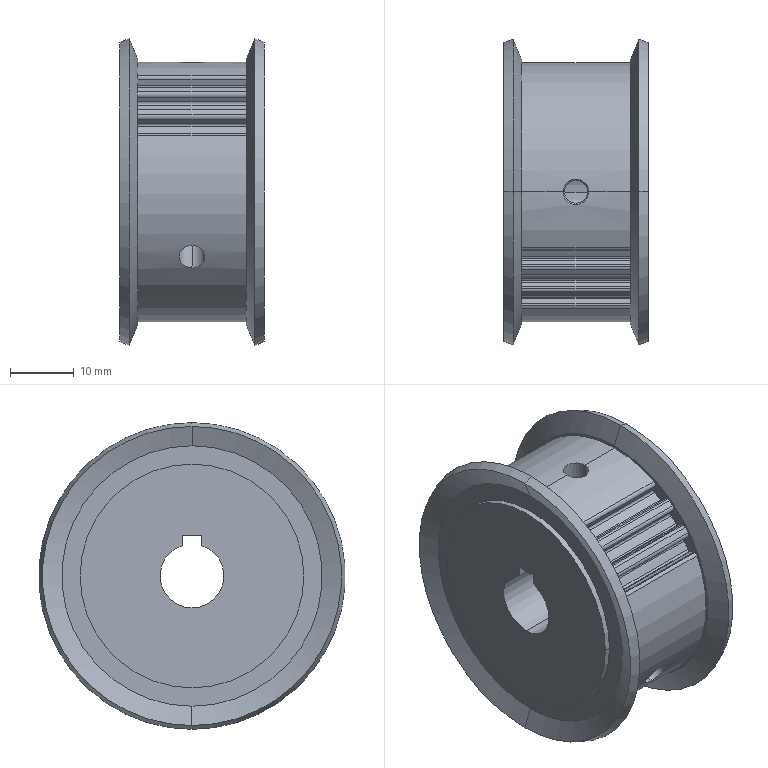Part | STEP file | Timing pulley TTPA26T5150-A-N10_MISUMI_default | 1 solid | 74 faces | box 22.642 x 48 x 48 mm | volume 27102 mm3 | cylinder 40 | plane 18 | cone 16 | commonest cylinder face diameters 0.8 x9 1.2 x9 40.6 x5 3.6 x4 4 x4 35 x4